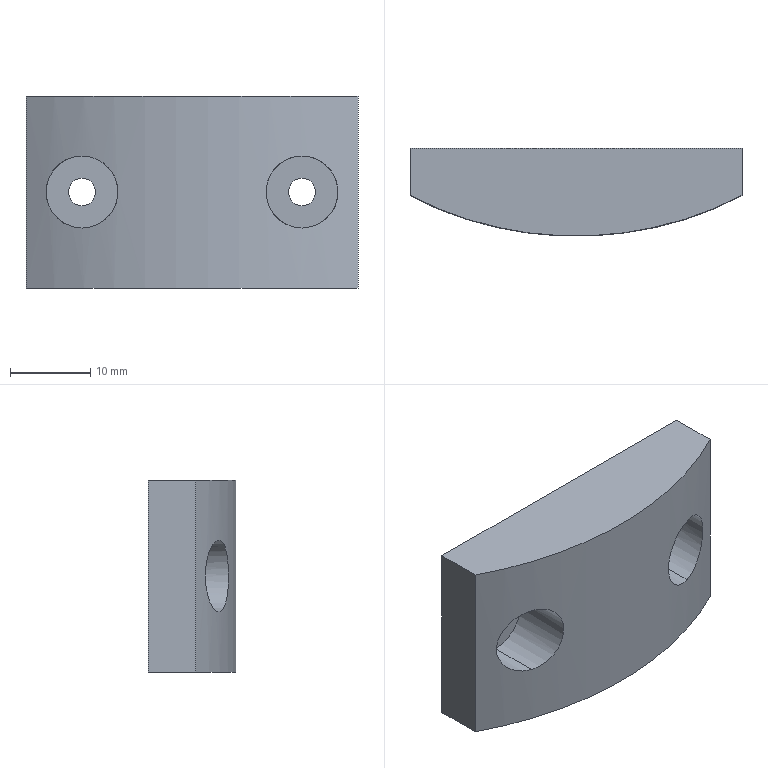Part | NX | features BREP 1 | 1 solid | 16 faces | box 41.5 x 11 x 24 mm | volume 8468 mm3 | cylinder 9 | plane 7 | commonest cylinder face diameters 3.4 x4 9 x4 90 x1
STEP:
#1=CARTESIAN_POINT('',(-13.75,-36.5,-4.5));
#2=VERTEX_POINT('',#1);
#3=CARTESIAN_POINT('',(-13.75,-36.5,4.5));
#4=VERTEX_POINT('',#3);
#5=CARTESIAN_POINT('',(-13.75,-36.5,0.));
#6=DIRECTION('',(0.,-1.,0.));
#7=DIRECTION('',(0.,0.,-1.));
#8=AXIS2_PLACEMENT_3D('',#5,#6,#7);
#9=CIRCLE('',#8,4.5);
#10=EDGE_CURVE('',#2,#4,#9,.T.);
#11=ORIENTED_EDGE('',*,*,#10,.T.);
#12=CARTESIAN_POINT('',(-13.75,-36.5,0.));
#13=DIRECTION('',(0.,-1.,0.));
#14=DIRECTION('',(0.,0.,-1.));
#15=AXIS2_PLACEMENT_3D('',#12,#13,#14);
#16=CIRCLE('',#15,4.5);
#17=EDGE_CURVE('',#4,#2,#16,.T.);
#18=ORIENTED_EDGE('',*,*,#17,.T.);
#19=EDGE_LOOP('',(#11,#18));
#20=FACE_BOUND('',#19,.T.);
#21=CARTESIAN_POINT('',(-13.75,-36.5,-1.7));
#22=VERTEX_POINT('',#21);
#23=CARTESIAN_POINT('',(-13.75,-36.5,1.7));
#24=VERTEX_POINT('',#23);
#25=CARTESIAN_POINT('',(-13.75,-36.5,0.));
#26=DIRECTION('',(0.,-1.,0.));
#27=DIRECTION('',(0.,0.,-1.));
#28=AXIS2_PLACEMENT_3D('',#25,#26,#27);
#29=CIRCLE('',#28,1.7);
#30=EDGE_CURVE('',#22,#24,#29,.T.);
#31=ORIENTED_EDGE('',*,*,#30,.F.);
#32=CARTESIAN_POINT('',(-13.75,-36.5,0.));
#33=DIRECTION('',(0.,-1.,0.));
#34=DIRECTION('',(0.,0.,-1.));
#35=AXIS2_PLACEMENT_3D('',#32,#33,#34);
#36=CIRCLE('',#35,1.7);
#37=EDGE_CURVE('',#24,#22,#36,.T.);
#38=ORIENTED_EDGE('',*,*,#37,.F.);
#39=EDGE_LOOP('',(#31,#38));
#40=FACE_BOUND('',#39,.T.);
#41=CARTESIAN_POINT('',(-12.05,-36.5,0.));
#42=DIRECTION('',(0.,1.,0.));
#43=DIRECTION('',(0.,0.,1.));
#44=AXIS2_PLACEMENT_3D('',#41,#42,#43);
#45=PLANE('',#44);
#46=ADVANCED_FACE('',(#20,#40),#45,.F.);
#47=CARTESIAN_POINT('',(-13.75,-34.,1.7));
#48=VERTEX_POINT('',#47);
#49=CARTESIAN_POINT('',(-13.75,-48.5,1.7));
#50=DIRECTION('',(0.,-1.,0.));
#51=VECTOR('',#50,1000.);
#52=LINE('',#49,#51);
#53=EDGE_CURVE('',#48,#24,#52,.T.);
#54=ORIENTED_EDGE('',*,*,#53,.F.);
#55=CARTESIAN_POINT('',(-13.75,-34.,-1.7));
#56=VERTEX_POINT('',#55);
#57=CARTESIAN_POINT('',(-13.75,-34.,0.));
#58=DIRECTION('',(0.,-1.,0.));
#59=DIRECTION('',(0.,0.,-1.));
#60=AXIS2_PLACEMENT_3D('',#57,#58,#59);
#61=CIRCLE('',#60,1.7);
#62=EDGE_CURVE('',#56,#48,#61,.T.);
#63=ORIENTED_EDGE('',*,*,#62,.F.);
#64=CARTESIAN_POINT('',(-13.75,-48.5,-1.7));
#65=DIRECTION('',(0.,-1.,0.));
#66=VECTOR('',#65,1000.);
#67=LINE('',#64,#66);
#68=EDGE_CURVE('',#56,#22,#67,.T.);
#69=ORIENTED_EDGE('',*,*,#68,.T.);
#70=ORIENTED_EDGE('',*,*,#30,.T.);
#71=EDGE_LOOP('',(#54,#63,#69,#70));
#72=FACE_BOUND('',#71,.T.);
#73=CARTESIAN_POINT('',(-13.75,-48.5,0.));
#74=DIRECTION('',(0.,-1.,0.));
#75=DIRECTION('',(0.,0.,-1.));
#76=AXIS2_PLACEMENT_3D('',#73,#74,#75);
#77=CYLINDRICAL_SURFACE('',#76,1.7);
#78=ADVANCED_FACE('',(#72),#77,.F.);
#79=CARTESIAN_POINT('',(-13.75,-42.848,4.5));
#80=VERTEX_POINT('',#79);
#81=CARTESIAN_POINT('',(-13.75,-48.5,4.5));
#82=DIRECTION('',(0.,-1.,0.));
#83=VECTOR('',#82,1000.);
#84=LINE('',#81,#83);
#85=EDGE_CURVE('',#4,#80,#84,.T.);
#86=ORIENTED_EDGE('',*,*,#85,.F.);
#87=ORIENTED_EDGE('',*,*,#10,.F.);
#88=CARTESIAN_POINT('',(-13.75,-42.848,-4.5));
#89=VERTEX_POINT('',#88);
#90=CARTESIAN_POINT('',(-13.75,-48.5,-4.5));
#91=DIRECTION('',(0.,-1.,0.));
#92=VECTOR('',#91,1000.);
#93=LINE('',#90,#92);
#94=EDGE_CURVE('',#2,#89,#93,.T.);
#95=ORIENTED_EDGE('',*,*,#94,.T.);
#96=CARTESIAN_POINT('',(-13.75,-42.848,-4.5));
#97=CARTESIAN_POINT('',(-13.123,-43.049,-4.5));
#98=CARTESIAN_POINT('',(-12.047,-43.368,-4.277));
#99=CARTESIAN_POINT('',(-10.,-43.893,-2.979));
#100=CARTESIAN_POINT('',(-8.747,-44.137,0.01097));
#101=CARTESIAN_POINT('',(-10.008,-43.891,2.987));
#102=CARTESIAN_POINT('',(-12.056,-43.365,4.28));
#103=CARTESIAN_POINT('',(-13.126,-43.048,4.5));
#104=CARTESIAN_POINT('',(-13.75,-42.848,4.5));
#105=B_SPLINE_CURVE_WITH_KNOTS('',3,(#96,#97,#98,#99,#100,#101,#102,#103,#104),.UNSPECIFIED.,.F.,.F.,(4,1,1,1,1,1,4),(0.,0.125,0.25,0.5,0.75,0.875,1.),.UNSPECIFIED.);
#106=EDGE_CURVE('',#80,#89,#105,.F.);
#107=ORIENTED_EDGE('',*,*,#106,.F.);
#108=EDGE_LOOP('',(#86,#87,#95,#107));
#109=FACE_BOUND('',#108,.T.);
#110=CARTESIAN_POINT('',(-13.75,-48.5,0.));
#111=DIRECTION('',(0.,-1.,0.));
#112=DIRECTION('',(0.,0.,-1.));
#113=AXIS2_PLACEMENT_3D('',#110,#111,#112);
#114=CYLINDRICAL_SURFACE('',#113,4.5);
#115=ADVANCED_FACE('',(#109),#114,.F.);
#116=CARTESIAN_POINT('',(13.75,-36.5,-4.5));
#117=VERTEX_POINT('',#116);
#118=CARTESIAN_POINT('',(13.75,-36.5,4.5));
#119=VERTEX_POINT('',#118);
#120=CARTESIAN_POINT('',(13.75,-36.5,0.));
#121=DIRECTION('',(0.,-1.,0.));
#122=DIRECTION('',(0.,0.,-1.));
#123=AXIS2_PLACEMENT_3D('',#120,#121,#122);
#124=CIRCLE('',#123,4.5);
#125=EDGE_CURVE('',#117,#119,#124,.T.);
#126=ORIENTED_EDGE('',*,*,#125,.T.);
#127=CARTESIAN_POINT('',(13.75,-36.5,0.));
#128=DIRECTION('',(0.,-1.,0.));
#129=DIRECTION('',(0.,0.,-1.));
#130=AXIS2_PLACEMENT_3D('',#127,#128,#129);
#131=CIRCLE('',#130,4.5);
#132=EDGE_CURVE('',#119,#117,#131,.T.);
#133=ORIENTED_EDGE('',*,*,#132,.T.);
#134=EDGE_LOOP('',(#126,#133));
#135=FACE_BOUND('',#134,.T.);
#136=CARTESIAN_POINT('',(13.75,-36.5,-1.7));
#137=VERTEX_POINT('',#136);
#138=CARTESIAN_POINT('',(13.75,-36.5,1.7));
#139=VERTEX_POINT('',#138);
#140=CARTESIAN_POINT('',(13.75,-36.5,0.));
#141=DIRECTION('',(0.,-1.,0.));
#142=DIRECTION('',(0.,0.,-1.));
#143=AXIS2_PLACEMENT_3D('',#140,#141,#142);
#144=CIRCLE('',#143,1.7);
#145=EDGE_CURVE('',#137,#139,#144,.T.);
#146=ORIENTED_EDGE('',*,*,#145,.F.);
#147=CARTESIAN_POINT('',(13.75,-36.5,0.));
#148=DIRECTION('',(0.,-1.,0.));
#149=DIRECTION('',(0.,0.,-1.));
#150=AXIS2_PLACEMENT_3D('',#147,#148,#149);
#151=CIRCLE('',#150,1.7);
#152=EDGE_CURVE('',#139,#137,#151,.T.);
#153=ORIENTED_EDGE('',*,*,#152,.F.);
#154=EDGE_LOOP('',(#146,#153));
#155=FACE_BOUND('',#154,.T.);
#156=CARTESIAN_POINT('',(15.45,-36.5,0.));
#157=DIRECTION('',(0.,1.,0.));
#158=DIRECTION('',(0.,0.,1.));
#159=AXIS2_PLACEMENT_3D('',#156,#157,#158);
#160=PLANE('',#159);
#161=ADVANCED_FACE('',(#135,#155),#160,.F.);
#162=CARTESIAN_POINT('',(13.75,-34.,1.7));
#163=VERTEX_POINT('',#162);
#164=CARTESIAN_POINT('',(13.75,-48.5,1.7));
#165=DIRECTION('',(0.,-1.,0.));
#166=VECTOR('',#165,1000.);
#167=LINE('',#164,#166);
#168=EDGE_CURVE('',#163,#139,#167,.T.);
#169=ORIENTED_EDGE('',*,*,#168,.F.);
#170=CARTESIAN_POINT('',(13.75,-34.,-1.7));
#171=VERTEX_POINT('',#170);
#172=CARTESIAN_POINT('',(13.75,-34.,0.));
#173=DIRECTION('',(0.,-1.,0.));
#174=DIRECTION('',(0.,0.,-1.));
#175=AXIS2_PLACEMENT_3D('',#172,#173,#174);
#176=CIRCLE('',#175,1.7);
#177=EDGE_CURVE('',#171,#163,#176,.T.);
#178=ORIENTED_EDGE('',*,*,#177,.F.);
#179=CARTESIAN_POINT('',(13.75,-48.5,-1.7));
#180=DIRECTION('',(0.,-1.,0.));
#181=VECTOR('',#180,1000.);
#182=LINE('',#179,#181);
#183=EDGE_CURVE('',#171,#137,#182,.T.);
#184=ORIENTED_EDGE('',*,*,#183,.T.);
#185=ORIENTED_EDGE('',*,*,#145,.T.);
#186=EDGE_LOOP('',(#169,#178,#184,#185));
#187=FACE_BOUND('',#186,.T.);
#188=CARTESIAN_POINT('',(13.75,-48.5,0.));
#189=DIRECTION('',(0.,-1.,0.));
#190=DIRECTION('',(0.,0.,-1.));
#191=AXIS2_PLACEMENT_3D('',#188,#189,#190);
#192=CYLINDRICAL_SURFACE('',#191,1.7);
#193=ADVANCED_FACE('',(#187),#192,.F.);
#194=CARTESIAN_POINT('',(13.75,-42.848,4.5));
#195=VERTEX_POINT('',#194);
#196=CARTESIAN_POINT('',(13.75,-48.5,4.5));
#197=DIRECTION('',(0.,-1.,0.));
#198=VECTOR('',#197,1000.);
#199=LINE('',#196,#198);
#200=EDGE_CURVE('',#119,#195,#199,.T.);
#201=ORIENTED_EDGE('',*,*,#200,.F.);
#202=ORIENTED_EDGE('',*,*,#125,.F.);
#203=CARTESIAN_POINT('',(13.75,-42.848,-4.5));
#204=VERTEX_POINT('',#203);
#205=CARTESIAN_POINT('',(13.75,-48.5,-4.5));
#206=DIRECTION('',(0.,-1.,0.));
#207=VECTOR('',#206,1000.);
#208=LINE('',#205,#207);
#209=EDGE_CURVE('',#117,#204,#208,.T.);
#210=ORIENTED_EDGE('',*,*,#209,.T.);
#211=CARTESIAN_POINT('',(13.75,-42.848,-4.5));
#212=CARTESIAN_POINT('',(14.001,-42.767,-4.5));
#213=CARTESIAN_POINT('',(14.649,-42.552,-4.437));
#214=CARTESIAN_POINT('',(15.418,-42.28,-4.217));
#215=CARTESIAN_POINT('',(16.349,-41.927,-3.707));
#216=CARTESIAN_POINT('',(16.866,-41.721,-3.282));
#217=CARTESIAN_POINT('',(17.536,-41.445,-2.493));
#218=CARTESIAN_POINT('',(17.902,-41.286,-1.802));
#219=CARTESIAN_POINT('',(18.199,-41.156,-0.8766));
#220=CARTESIAN_POINT('',(18.276,-41.121,0.01186));
#221=CARTESIAN_POINT('',(18.195,-41.158,0.8941));
#222=CARTESIAN_POINT('',(17.895,-41.289,1.817));
#223=CARTESIAN_POINT('',(17.528,-41.448,2.502));
#224=CARTESIAN_POINT('',(16.975,-41.676,3.16));
#225=CARTESIAN_POINT('',(16.594,-41.829,3.497));
#226=CARTESIAN_POINT('',(16.184,-41.989,3.792));
#227=CARTESIAN_POINT('',(15.899,-42.098,3.961));
#228=CARTESIAN_POINT('',(15.273,-42.331,4.258));
#229=CARTESIAN_POINT('',(14.626,-42.56,4.437));
#230=CARTESIAN_POINT('',(14.045,-42.753,4.5));
#231=CARTESIAN_POINT('',(13.75,-42.848,4.5));
#232=B_SPLINE_CURVE_WITH_KNOTS('',3,(#211,#212,#213,#214,#215,#216,#217,#218,#219,#220,#221,#222,#223,#224,#225,#226,#227,#228,#229,#230,#231),.UNSPECIFIED.,.F.,.F.,(4,1,1,1,1,1,1,1,1,1,1,1,1,1,1,1,1,1,4),(0.,0.0625,0.125,0.1875,0.25,0.3125,0.375,0.4375,0.5,0.5625,0.625,0.6875,0.75,0.7812,0.8125,0.8438,0.875,0.9375,1.),.UNSPECIFIED.);
#233=EDGE_CURVE('',#195,#204,#232,.F.);
#234=ORIENTED_EDGE('',*,*,#233,.F.);
#235=EDGE_LOOP('',(#201,#202,#210,#234));
#236=FACE_BOUND('',#235,.T.);
#237=CARTESIAN_POINT('',(13.75,-48.5,0.));
#238=DIRECTION('',(0.,-1.,0.));
#239=DIRECTION('',(0.,0.,-1.));
#240=AXIS2_PLACEMENT_3D('',#237,#238,#239);
#241=CYLINDRICAL_SURFACE('',#240,4.5);
#242=ADVANCED_FACE('',(#236),#241,.F.);
#243=CARTESIAN_POINT('',(-20.75,-39.93,-12.));
#244=VERTEX_POINT('',#243);
#245=CARTESIAN_POINT('',(20.75,-39.93,-12.));
#246=VERTEX_POINT('',#245);
#247=CARTESIAN_POINT('',(0.,0.,-12.));
#248=DIRECTION('',(0.,0.,1.));
#249=DIRECTION('',(1.,0.,0.));
#250=AXIS2_PLACEMENT_3D('',#247,#248,#249);
#251=CIRCLE('',#250,45.);
#252=EDGE_CURVE('',#244,#246,#251,.T.);
#253=ORIENTED_EDGE('',*,*,#252,.F.);
#254=CARTESIAN_POINT('',(-20.75,-34.,-12.));
#255=VERTEX_POINT('',#254);
#256=CARTESIAN_POINT('',(-20.75,-39.93,-12.));
#257=DIRECTION('',(0.,-1.,0.));
#258=VECTOR('',#257,1000.);
#259=LINE('',#256,#258);
#260=EDGE_CURVE('',#255,#244,#259,.T.);
#261=ORIENTED_EDGE('',*,*,#260,.F.);
#262=CARTESIAN_POINT('',(20.75,-34.,-12.));
#263=VERTEX_POINT('',#262);
#264=CARTESIAN_POINT('',(-20.75,-34.,-12.));
#265=DIRECTION('',(-1.,0.,0.));
#266=VECTOR('',#265,1000.);
#267=LINE('',#264,#266);
#268=EDGE_CURVE('',#263,#255,#267,.T.);
#269=ORIENTED_EDGE('',*,*,#268,.F.);
#270=CARTESIAN_POINT('',(20.75,-34.,-12.));
#271=DIRECTION('',(0.,1.,0.));
#272=VECTOR('',#271,1000.);
#273=LINE('',#270,#272);
#274=EDGE_CURVE('',#246,#263,#273,.T.);
#275=ORIENTED_EDGE('',*,*,#274,.F.);
#276=EDGE_LOOP('',(#253,#261,#269,#275));
#277=FACE_BOUND('',#276,.T.);
#278=CARTESIAN_POINT('',(0.,0.,-12.));
#279=DIRECTION('',(0.,0.,1.));
#280=DIRECTION('',(1.,0.,0.));
#281=AXIS2_PLACEMENT_3D('',#278,#279,#280);
#282=PLANE('',#281);
#283=ADVANCED_FACE('',(#277),#282,.F.);
#284=CARTESIAN_POINT('',(-20.75,-39.93,12.));
#285=VERTEX_POINT('',#284);
#286=CARTESIAN_POINT('',(20.75,-39.93,12.));
#287=VERTEX_POINT('',#286);
#288=CARTESIAN_POINT('',(0.,0.,12.));
#289=DIRECTION('',(0.,0.,1.));
#290=DIRECTION('',(1.,0.,0.));
#291=AXIS2_PLACEMENT_3D('',#288,#289,#290);
#292=CIRCLE('',#291,45.);
#293=EDGE_CURVE('',#285,#287,#292,.T.);
#294=ORIENTED_EDGE('',*,*,#293,.T.);
#295=CARTESIAN_POINT('',(20.75,-34.,12.));
#296=VERTEX_POINT('',#295);
#297=CARTESIAN_POINT('',(20.75,-34.,12.));
#298=DIRECTION('',(0.,1.,0.));
#299=VECTOR('',#298,1000.);
#300=LINE('',#297,#299);
#301=EDGE_CURVE('',#287,#296,#300,.T.);
#302=ORIENTED_EDGE('',*,*,#301,.T.);
#303=CARTESIAN_POINT('',(-20.75,-34.,12.));
#304=VERTEX_POINT('',#303);
#305=CARTESIAN_POINT('',(-20.75,-34.,12.));
#306=DIRECTION('',(-1.,0.,0.));
#307=VECTOR('',#306,1000.);
#308=LINE('',#305,#307);
#309=EDGE_CURVE('',#296,#304,#308,.T.);
#310=ORIENTED_EDGE('',*,*,#309,.T.);
#311=CARTESIAN_POINT('',(-20.75,-39.93,12.));
#312=DIRECTION('',(0.,-1.,0.));
#313=VECTOR('',#312,1000.);
#314=LINE('',#311,#313);
#315=EDGE_CURVE('',#304,#285,#314,.T.);
#316=ORIENTED_EDGE('',*,*,#315,.T.);
#317=EDGE_LOOP('',(#294,#302,#310,#316));
#318=FACE_BOUND('',#317,.T.);
#319=CARTESIAN_POINT('',(0.,0.,12.));
#320=DIRECTION('',(0.,0.,1.));
#321=DIRECTION('',(1.,0.,0.));
#322=AXIS2_PLACEMENT_3D('',#319,#320,#321);
#323=PLANE('',#322);
#324=ADVANCED_FACE('',(#318),#323,.T.);
#325=ORIENTED_EDGE('',*,*,#260,.T.);
#326=CARTESIAN_POINT('',(-20.75,-39.93,12.));
#327=DIRECTION('',(0.,0.,-1.));
#328=VECTOR('',#327,1000.);
#329=LINE('',#326,#328);
#330=EDGE_CURVE('',#285,#244,#329,.T.);
#331=ORIENTED_EDGE('',*,*,#330,.F.);
#332=ORIENTED_EDGE('',*,*,#315,.F.);
#333=CARTESIAN_POINT('',(-20.75,-34.,12.));
#334=DIRECTION('',(0.,0.,-1.));
#335=VECTOR('',#334,1000.);
#336=LINE('',#333,#335);
#337=EDGE_CURVE('',#304,#255,#336,.T.);
#338=ORIENTED_EDGE('',*,*,#337,.T.);
#339=EDGE_LOOP('',(#325,#331,#332,#338));
#340=FACE_BOUND('',#339,.T.);
#341=CARTESIAN_POINT('',(-20.75,-39.93,12.));
#342=DIRECTION('',(1.,0.,0.));
#343=DIRECTION('',(0.,0.,-1.));
#344=AXIS2_PLACEMENT_3D('',#341,#342,#343);
#345=PLANE('',#344);
#346=ADVANCED_FACE('',(#340),#345,.F.);
#347=ORIENTED_EDGE('',*,*,#268,.T.);
#348=ORIENTED_EDGE('',*,*,#337,.F.);
#349=ORIENTED_EDGE('',*,*,#309,.F.);
#350=CARTESIAN_POINT('',(20.75,-34.,12.));
#351=DIRECTION('',(0.,0.,-1.));
#352=VECTOR('',#351,1000.);
#353=LINE('',#350,#352);
#354=EDGE_CURVE('',#296,#263,#353,.T.);
#355=ORIENTED_EDGE('',*,*,#354,.T.);
#356=EDGE_LOOP('',(#347,#348,#349,#355));
#357=FACE_BOUND('',#356,.T.);
#358=ORIENTED_EDGE('',*,*,#177,.T.);
#359=CARTESIAN_POINT('',(13.75,-34.,0.));
#360=DIRECTION('',(0.,-1.,0.));
#361=DIRECTION('',(0.,0.,-1.));
#362=AXIS2_PLACEMENT_3D('',#359,#360,#361);
#363=CIRCLE('',#362,1.7);
#364=EDGE_CURVE('',#163,#171,#363,.T.);
#365=ORIENTED_EDGE('',*,*,#364,.T.);
#366=EDGE_LOOP('',(#358,#365));
#367=FACE_BOUND('',#366,.T.);
#368=ORIENTED_EDGE('',*,*,#62,.T.);
#369=CARTESIAN_POINT('',(-13.75,-34.,0.));
#370=DIRECTION('',(0.,-1.,0.));
#371=DIRECTION('',(0.,0.,-1.));
#372=AXIS2_PLACEMENT_3D('',#369,#370,#371);
#373=CIRCLE('',#372,1.7);
#374=EDGE_CURVE('',#48,#56,#373,.T.);
#375=ORIENTED_EDGE('',*,*,#374,.T.);
#376=EDGE_LOOP('',(#368,#375));
#377=FACE_BOUND('',#376,.T.);
#378=CARTESIAN_POINT('',(-20.75,-34.,12.));
#379=DIRECTION('',(0.,-1.,0.));
#380=DIRECTION('',(1.,0.,0.));
#381=AXIS2_PLACEMENT_3D('',#378,#379,#380);
#382=PLANE('',#381);
#383=ADVANCED_FACE('',(#357,#367,#377),#382,.F.);
#384=ORIENTED_EDGE('',*,*,#274,.T.);
#385=ORIENTED_EDGE('',*,*,#354,.F.);
#386=ORIENTED_EDGE('',*,*,#301,.F.);
#387=CARTESIAN_POINT('',(20.75,-39.93,12.));
#388=DIRECTION('',(0.,0.,-1.));
#389=VECTOR('',#388,1000.);
#390=LINE('',#387,#389);
#391=EDGE_CURVE('',#287,#246,#390,.T.);
#392=ORIENTED_EDGE('',*,*,#391,.T.);
#393=EDGE_LOOP('',(#384,#385,#386,#392));
#394=FACE_BOUND('',#393,.T.);
#395=CARTESIAN_POINT('',(20.75,-34.,12.));
#396=DIRECTION('',(-1.,0.,0.));
#397=DIRECTION('',(0.,0.,1.));
#398=AXIS2_PLACEMENT_3D('',#395,#396,#397);
#399=PLANE('',#398);
#400=ADVANCED_FACE('',(#394),#399,.F.);
#401=ORIENTED_EDGE('',*,*,#252,.T.);
#402=ORIENTED_EDGE('',*,*,#391,.F.);
#403=ORIENTED_EDGE('',*,*,#293,.F.);
#404=ORIENTED_EDGE('',*,*,#330,.T.);
#405=EDGE_LOOP('',(#401,#402,#403,#404));
#406=FACE_BOUND('',#405,.T.);
#407=CARTESIAN_POINT('',(13.75,-42.848,-4.5));
#408=CARTESIAN_POINT('',(12.601,-43.217,-4.5));
#409=CARTESIAN_POINT('',(10.28,-43.838,-3.584));
#410=CARTESIAN_POINT('',(8.735,-44.139,-0.005547));
#411=CARTESIAN_POINT('',(10.278,-43.839,3.584));
#412=CARTESIAN_POINT('',(12.597,-43.218,4.5));
#413=CARTESIAN_POINT('',(13.75,-42.848,4.5));
#414=B_SPLINE_CURVE_WITH_KNOTS('',3,(#407,#408,#409,#410,#411,#412,#413),.UNSPECIFIED.,.F.,.F.,(4,1,1,1,4),(0.,0.25,0.5,0.75,1.),.UNSPECIFIED.);
#415=EDGE_CURVE('',#204,#195,#414,.T.);
#416=ORIENTED_EDGE('',*,*,#415,.T.);
#417=ORIENTED_EDGE('',*,*,#233,.T.);
#418=EDGE_LOOP('',(#416,#417));
#419=FACE_BOUND('',#418,.T.);
#420=CARTESIAN_POINT('',(-13.75,-42.848,-4.5));
#421=CARTESIAN_POINT('',(-14.909,-42.476,-4.5));
#422=CARTESIAN_POINT('',(-17.195,-41.618,-3.599));
#423=CARTESIAN_POINT('',(-18.777,-40.891,-0.01078));
#424=CARTESIAN_POINT('',(-17.197,-41.617,3.601));
#425=CARTESIAN_POINT('',(-14.913,-42.474,4.5));
#426=CARTESIAN_POINT('',(-13.75,-42.848,4.5));
#427=B_SPLINE_CURVE_WITH_KNOTS('',3,(#420,#421,#422,#423,#424,#425,#426),.UNSPECIFIED.,.F.,.F.,(4,1,1,1,4),(0.,0.25,0.5,0.75,1.),.UNSPECIFIED.);
#428=EDGE_CURVE('',#89,#80,#427,.T.);
#429=ORIENTED_EDGE('',*,*,#428,.T.);
#430=ORIENTED_EDGE('',*,*,#106,.T.);
#431=EDGE_LOOP('',(#429,#430));
#432=FACE_BOUND('',#431,.T.);
#433=CARTESIAN_POINT('',(0.,0.,12.));
#434=DIRECTION('',(0.,0.,-1.));
#435=DIRECTION('',(-1.,0.,0.));
#436=AXIS2_PLACEMENT_3D('',#433,#434,#435);
#437=CYLINDRICAL_SURFACE('',#436,45.);
#438=ADVANCED_FACE('',(#406,#419,#432),#437,.T.);
#439=ORIENTED_EDGE('',*,*,#132,.F.);
#440=ORIENTED_EDGE('',*,*,#200,.T.);
#441=ORIENTED_EDGE('',*,*,#415,.F.);
#442=ORIENTED_EDGE('',*,*,#209,.F.);
#443=EDGE_LOOP('',(#439,#440,#441,#442));
#444=FACE_BOUND('',#443,.T.);
#445=CARTESIAN_POINT('',(13.75,-48.5,0.));
#446=DIRECTION('',(0.,-1.,0.));
#447=DIRECTION('',(0.,0.,-1.));
#448=AXIS2_PLACEMENT_3D('',#445,#446,#447);
#449=CYLINDRICAL_SURFACE('',#448,4.5);
#450=ADVANCED_FACE('',(#444),#449,.F.);
#451=ORIENTED_EDGE('',*,*,#364,.F.);
#452=ORIENTED_EDGE('',*,*,#168,.T.);
#453=ORIENTED_EDGE('',*,*,#152,.T.);
#454=ORIENTED_EDGE('',*,*,#183,.F.);
#455=EDGE_LOOP('',(#451,#452,#453,#454));
#456=FACE_BOUND('',#455,.T.);
#457=CARTESIAN_POINT('',(13.75,-48.5,0.));
#458=DIRECTION('',(0.,-1.,0.));
#459=DIRECTION('',(0.,0.,-1.));
#460=AXIS2_PLACEMENT_3D('',#457,#458,#459);
#461=CYLINDRICAL_SURFACE('',#460,1.7);
#462=ADVANCED_FACE('',(#456),#461,.F.);
#463=ORIENTED_EDGE('',*,*,#17,.F.);
#464=ORIENTED_EDGE('',*,*,#85,.T.);
#465=ORIENTED_EDGE('',*,*,#428,.F.);
#466=ORIENTED_EDGE('',*,*,#94,.F.);
#467=EDGE_LOOP('',(#463,#464,#465,#466));
#468=FACE_BOUND('',#467,.T.);
#469=CARTESIAN_POINT('',(-13.75,-48.5,0.));
#470=DIRECTION('',(0.,-1.,0.));
#471=DIRECTION('',(0.,0.,-1.));
#472=AXIS2_PLACEMENT_3D('',#469,#470,#471);
#473=CYLINDRICAL_SURFACE('',#472,4.5);
#474=ADVANCED_FACE('',(#468),#473,.F.);
#475=ORIENTED_EDGE('',*,*,#374,.F.);
#476=ORIENTED_EDGE('',*,*,#53,.T.);
#477=ORIENTED_EDGE('',*,*,#37,.T.);
#478=ORIENTED_EDGE('',*,*,#68,.F.);
#479=EDGE_LOOP('',(#475,#476,#477,#478));
#480=FACE_BOUND('',#479,.T.);
#481=CARTESIAN_POINT('',(-13.75,-48.5,0.));
#482=DIRECTION('',(0.,-1.,0.));
#483=DIRECTION('',(0.,0.,-1.));
#484=AXIS2_PLACEMENT_3D('',#481,#482,#483);
#485=CYLINDRICAL_SURFACE('',#484,1.7);
#486=ADVANCED_FACE('',(#480),#485,.F.);
#487=CLOSED_SHELL('',(#46,#78,#115,#161,#193,#242,#283,#324,#346,#383,#400,#438,#450,#462,#474,#486));
#488=MANIFOLD_SOLID_BREP('',#487);
#489=(LENGTH_UNIT()NAMED_UNIT(*)SI_UNIT(.MILLI.,.METRE.));
#490=UNCERTAINTY_MEASURE_WITH_UNIT(LENGTH_MEASURE(0.0508),#489,'','');
#491=(NAMED_UNIT(*)PLANE_ANGLE_UNIT()SI_UNIT($,.RADIAN.));
#492=(NAMED_UNIT(*)SI_UNIT($,.STERADIAN.)SOLID_ANGLE_UNIT());
#493=(GEOMETRIC_REPRESENTATION_CONTEXT(3)GLOBAL_UNCERTAINTY_ASSIGNED_CONTEXT((#490))GLOBAL_UNIT_ASSIGNED_CONTEXT((#489,#491,#492))REPRESENTATION_CONTEXT('',''));
#494=ADVANCED_BREP_SHAPE_REPRESENTATION('',(#488),#493);